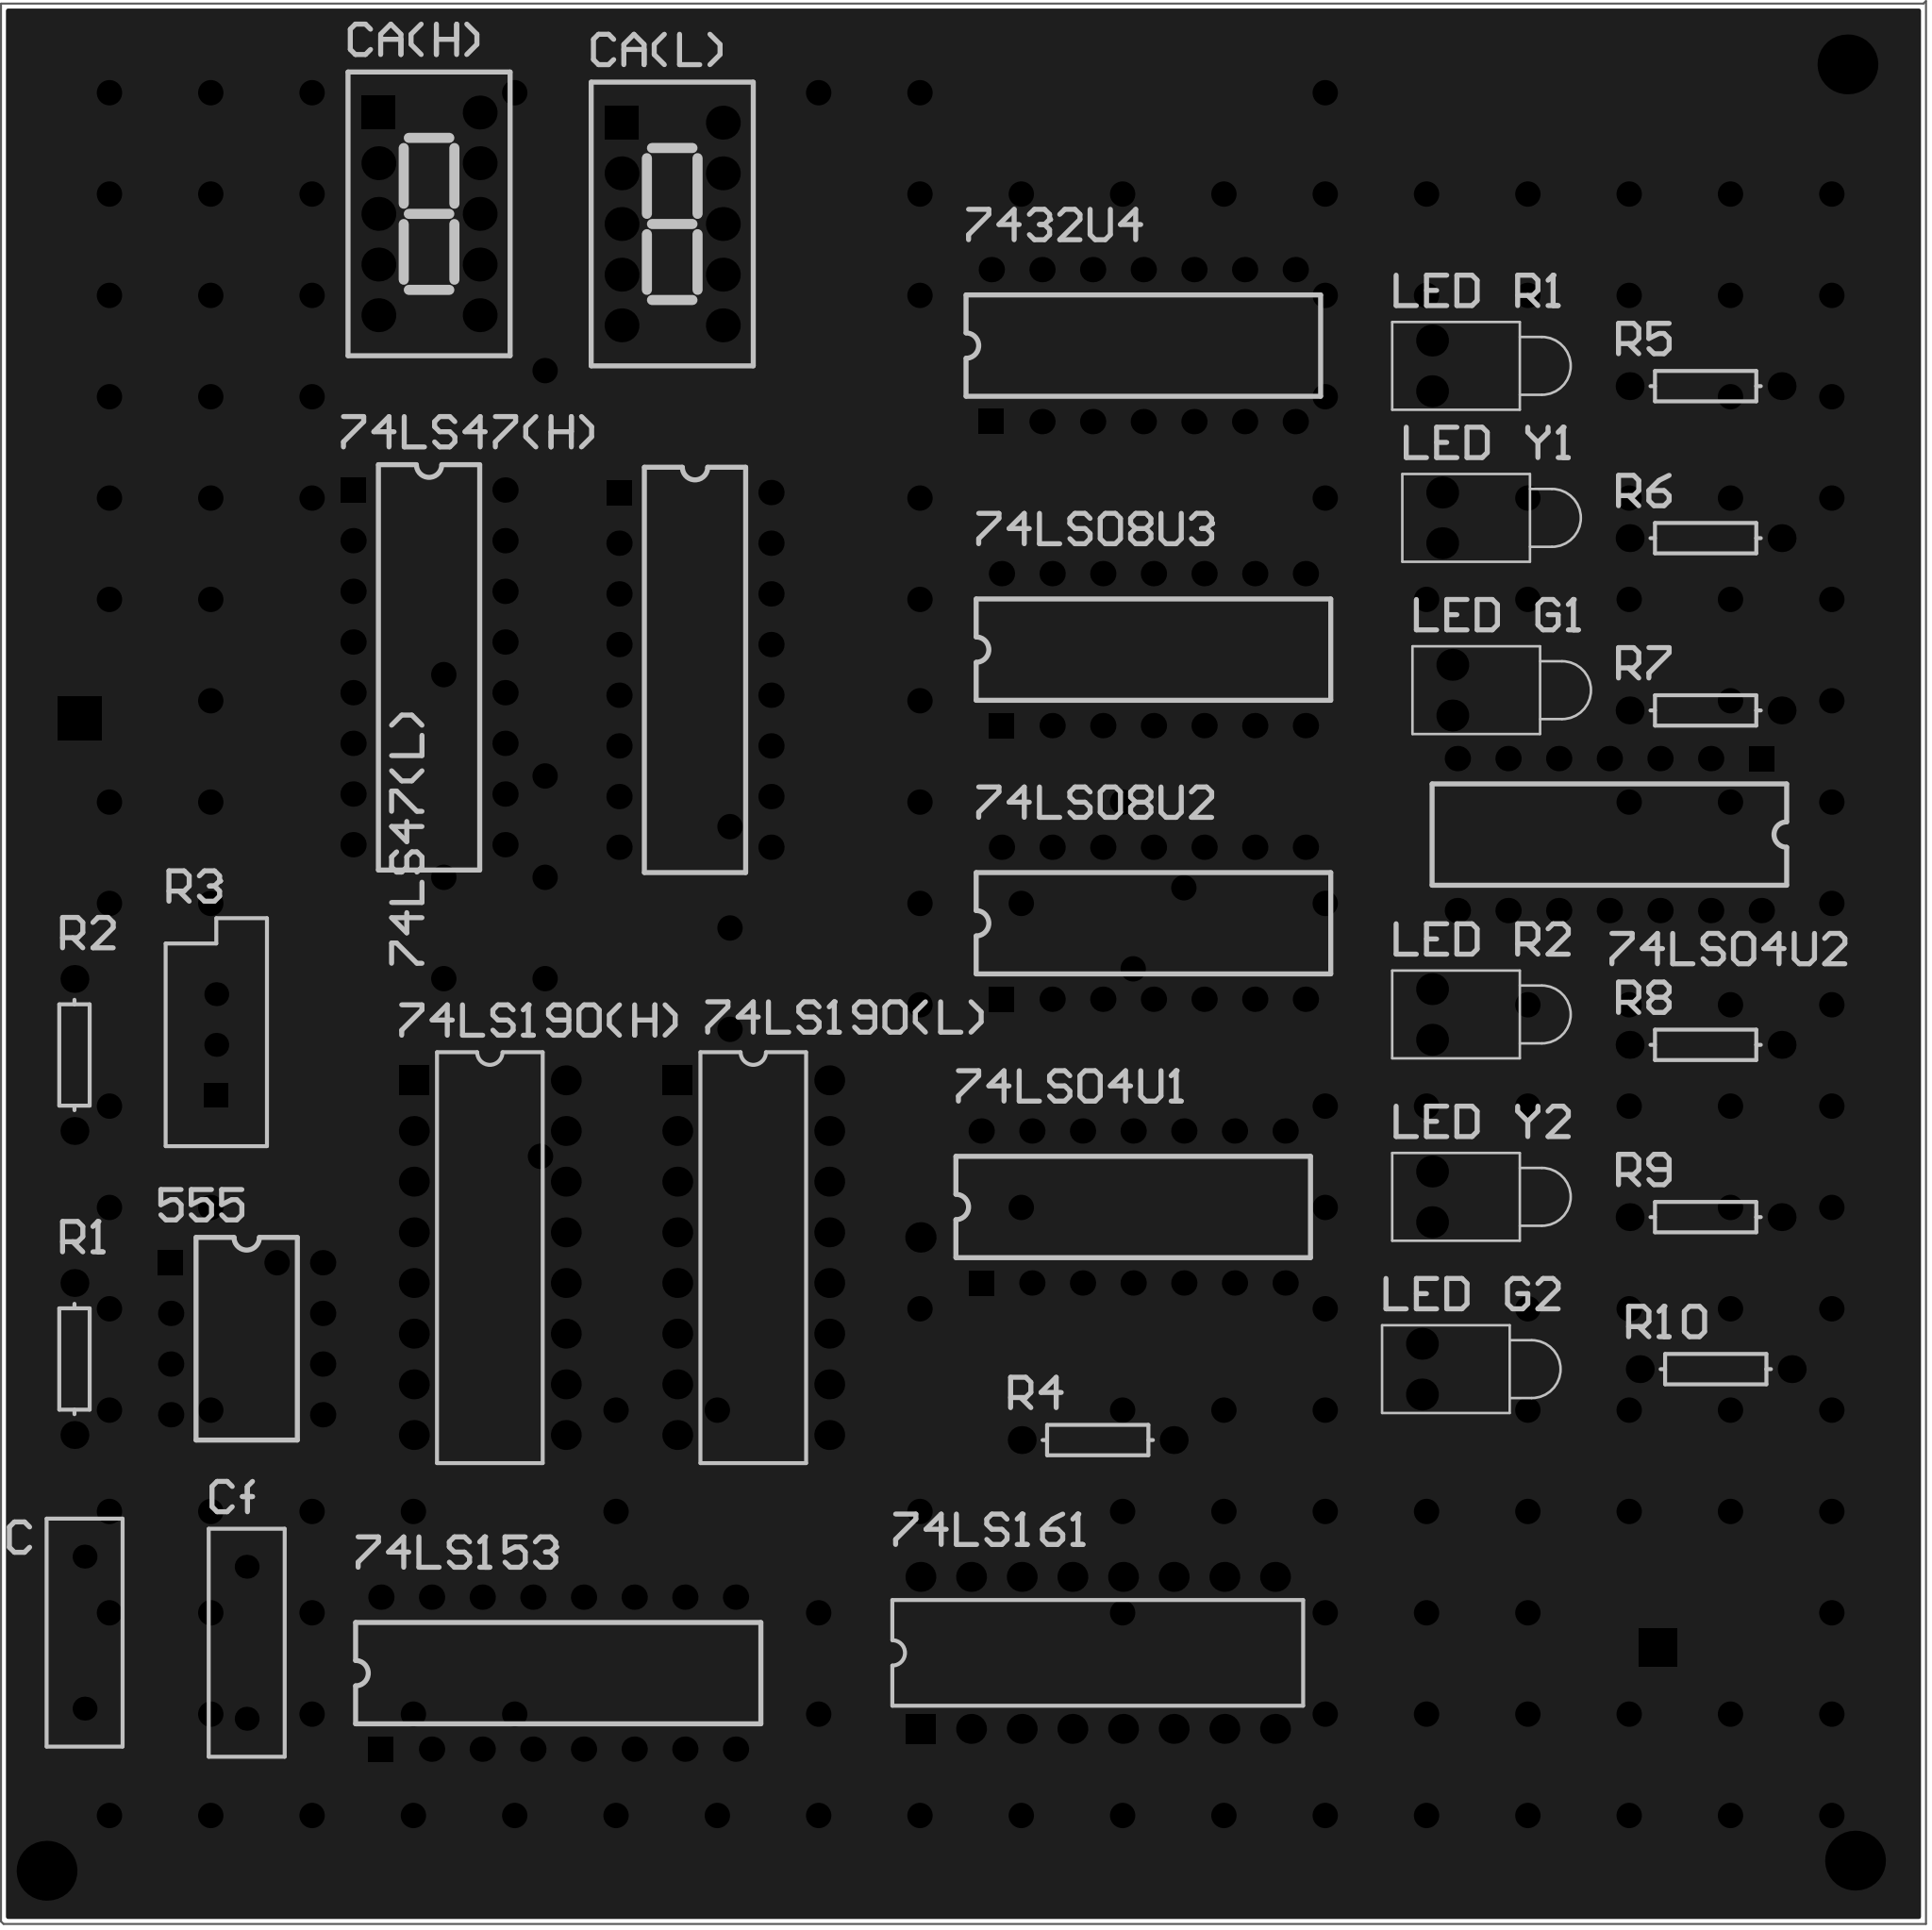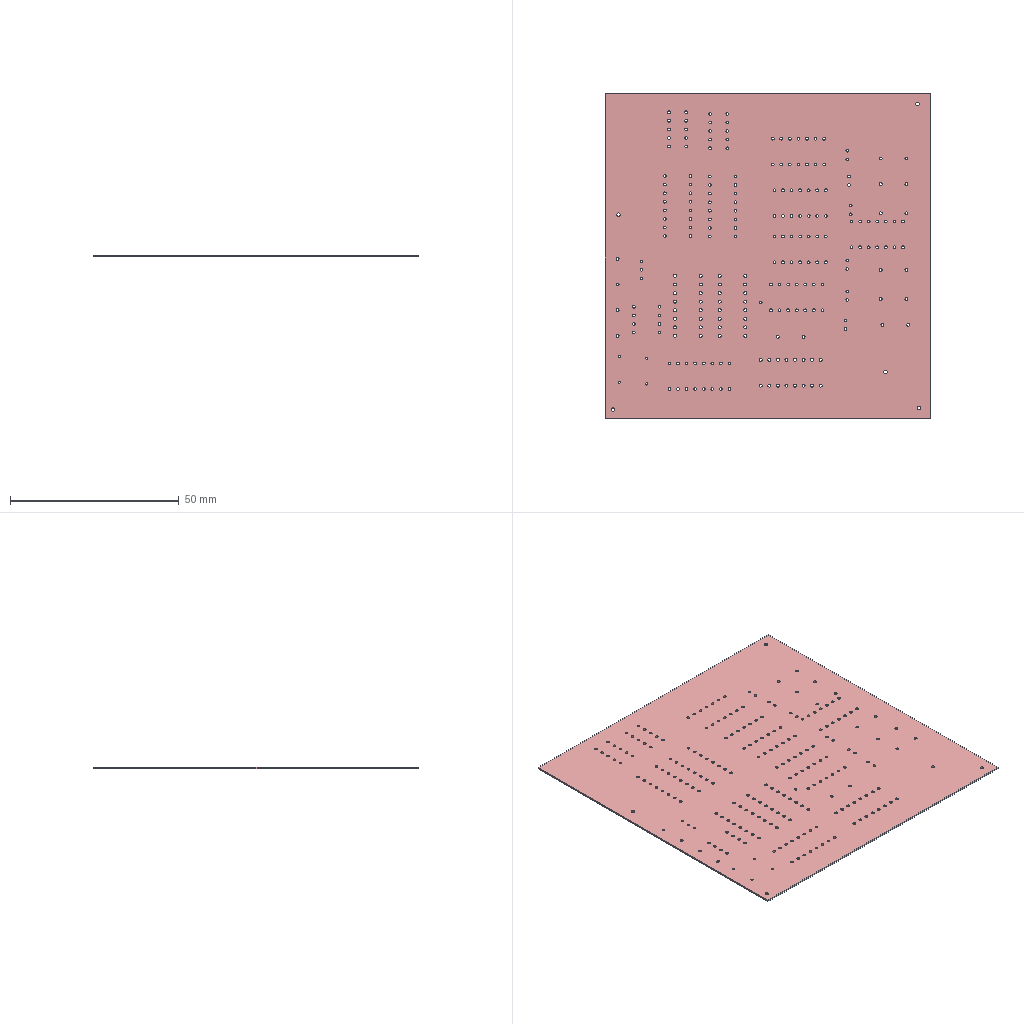Circuit board layout | Altium Designer | box 96.5 x 96.4 x 0.5 mm
Layer stack:
# Altium Designer layer stack of  (unit mm; dielectric type: 0 none, 1 core, 2 prepreg, 3 surface material)
index,name,kind,layer,copper_thickness_mm,dielectric_type,dielectric_thickness_mm,dielectric_material,dielectric_constant
0,Top Paste Mask Layer,other,,,,,,
1,Top Silkscreen Layer,other,,,,,,
2,Top Solder Mask Layer,dielectric,,,3,0.0356,FR-4,4.8
3,Top Layer,copper,Top Layer,0.0356,,,,
4,Substrate1,dielectric,,,3,0.32,FR-4,4.8
5,Bottom Layer,copper,Bottom Layer,0.0356,,,,
6,Bottom Solder Mask Layer,dielectric,,,3,0.0356,FR-4,4.8
7,Bottom Silkscreen Layer,other,,,,,,
8,Bottom Paste Mask Layer,other,,,,,,
# drill layer pairs: low layer,high layer
drill_pair,Top Layer,Bottom Layer
Part placement:
Designator,Comment,Layer,Footprint,Center-X(mm),Center-Y(mm),Rotation
R10,Res1,TopLayer,AXIAL-0.3,172.339,114.3,0
R9,Res1,TopLayer,AXIAL-0.3,171.831,121.92,0
R8,Res1,TopLayer,AXIAL-0.3,171.831,130.556,0
R7,Res1,TopLayer,AXIAL-0.3,171.831,147.32,0
R6,Res1,TopLayer,AXIAL-0.3,171.831,155.956,0
R5,Res1,TopLayer,AXIAL-0.3,171.831,163.576,0
R4,Res1,TopLayer,AXIAL-0.3,141.351,110.744,180
R3,RPot,TopLayer,VR5,97.155,130.556,90
R2,Res1,TopLayer,AXIAL-0.3,90.043,130.048,90
R1,Res1,TopLayer,AXIAL-0.3,90.043,114.808,90
LED Y2,LED1,TopLayer,LED-1,158.115,122.936,0
LED Y1,LED1,TopLayer,LED-1,158.623,156.972,0
LED R2,LED1,TopLayer,LED-1,158.115,132.08,0
LED R1,LED1,TopLayer,LED-1,158.115,164.592,0
LED G2,LED1,TopLayer,LED-1,157.607,114.3,0
LED G1,LED1,TopLayer,LED-1,159.131,148.336,0
C,Cap,TopLayer,RAD-0.3,90.551,101.092,90
Cf,Cap,TopLayer,RAD-0.3,98.679,100.584,90
7432U4,7432,TopLayer,DIP14,143.637,165.608,90
555,555,TopLayer,DIP8,98.679,115.824,0
74LS190(L),SN74LS190,TopLayer,DIP-16,124.079,119.888,270
74LS190(H),SN74LS190,TopLayer,DIP-16,110.871,119.888,270
74LS161,74LS161A,TopLayer,DIP-16,141.351,100.076,0
74LS153,SN74LS153,TopLayer,DIP16,114.3,99.06,90
74LS47(H),SN7447A,TopLayer,DIP16,107.823,149.479,0
74LS08U3,74LS08,TopLayer,DIP14,144.145,150.368,90
74LS08U2,74LS08,TopLayer,DIP14,144.145,136.652,90
74LS04U1,74LS04,TopLayer,DIP14,143.129,122.428,90
74LS04U2,74LS04,TopLayer,DIP14,167.005,141.097,270
74LS47(L),SN7447A,TopLayer,DIP16,121.158,149.352,0
CA(H),Dpy Red-CA,TopLayer,SMG_0.36-1P,107.823,172.212,0
CA(L),Dpy Red-CA,TopLayer,SMG_0.36-1P,120.015,171.704,0
Pad and via stacks:
# Altium Designer via and pad stacks of  (unit mm). Each distinct definition once, with the count of objects using it.
# via: kind,start_layer,end_layer,hole_mm,diameter_mm,mode(0 simple;1 top-mid-bottom;2 full stack),diameter_per_layer,count,example_net
# pad: kind,layer,hole_mm,hole_type(0 round;1 square;2 slot),plating,top_size,top_shape(1 round;2 rect;3 octagon;9 rounded rect),mid_size,bottom_size,mode,footprint,size_per_layer,count,example
pad,Multi-Layer,1,0,plated,1.9x1.9,2,1.9x1.9,1.9x1.9,0,,,1,3
pad,Multi-Layer,1,0,plated,2.2x2.2,2,2.2x2.2,2.2x2.2,0,,,1,2
pad,Multi-Layer,0.762,0,plated,1.524x1.524,1,1.524x1.524,1.524x1.524,0,,,1,1
pad,Multi-Layer,1,0,unplated,3x3,1,3x3,3x3,0,,,3,12
pad,Multi-Layer,0.85,0,plated,1.4x1.4,1,1.4x1.4,1.4x1.4,0,AXIAL-0.3,,18,R10.2
pad,Multi-Layer,0.7,0,plated,1.2x1.2,2,1.2x1.2,1.2x1.2,0,VR5,,1,R3.1
pad,Multi-Layer,0.7,0,plated,1.2x1.2,1,1.2x1.2,1.2x1.2,0,VR5,,2,R3.2
pad,Multi-Layer,0.8,0,plated,1.6x1.6,1,1.6x1.6,1.6x1.6,0,LED-1,,12,LED Y2.1
pad,Multi-Layer,0.7,0,plated,1.2x1.2,1,1.2x1.2,1.2x1.2,0,RAD-0.3,,4,C.2
pad,Multi-Layer,0.8128,0,plated,1.27x1.27,1,1.27x1.27,1.27x1.27,0,DIP14,,65,7432U4.14
pad,Multi-Layer,0.8128,0,plated,1.27x1.27,2,1.27x1.27,1.27x1.27,0,DIP14,,5,7432U4.1
pad,Multi-Layer,0.8128,0,plated,1.27x1.27,2,1.27x1.27,1.27x1.27,0,DIP8,,1,555.1
pad,Multi-Layer,0.8128,0,plated,1.27x1.27,1,1.27x1.27,1.27x1.27,0,DIP8,,7,555.2
pad,Multi-Layer,0.9,0,plated,1.5x1.5,1,1.5x1.5,1.5x1.5,0,DIP-16,,45,74LS190(L).9
pad,Multi-Layer,0.9,0,plated,1.5x1.5,2,1.5x1.5,1.5x1.5,0,DIP-16,,3,74LS190(L).1
pad,Multi-Layer,0.8128,0,plated,1.27x1.27,2,1.27x1.27,1.27x1.27,0,DIP16,,3,74LS153.1
pad,Multi-Layer,0.8128,0,plated,1.27x1.27,1,1.27x1.27,1.27x1.27,0,DIP16,,45,74LS153.2
pad,Multi-Layer,0.8,0,plated,1.7x1.7,1,1.7x1.7,1.7x1.7,0,SMG 0.36-1P,,18,CA(H).10
pad,Multi-Layer,0.8,0,plated,1.7x1.7,2,1.7x1.7,1.7x1.7,0,SMG 0.36-1P,,2,CA(H).1
via,Top Layer,Bottom Layer,0.7112,1.27,0,,172,$2N1342
Copper pours:
name,layer,net,type(0 solid;1 hatched;2 none)
Top Layer-GND,Top Layer,GND,0
Bottom Layer-GND,Bottom Layer,GND,0
Design rules, without the lines most boards share:
# Altium Designer design rules of  (exported by Altium Designer, unit mm)
# columns: name | kind | enabled | priority | scope1 | scope2 | descriptor | typed fields (field=value)
ComponentClearance_1 | 24 | enabled | 1 | All | All | Component Clearance Constraint ( Horizontal Gap = 10mil, Vertical Gap = 10mil ) (All),(All)  | gap=0.254
Plane_PlaneConnect | 0 | disabled | 1 | All | All | Clearance Constraint (Gap=10mil) (Disabled)(All),(All) | gap=0.254
Plane_PlaneConnect_1 | 63 | disabled | 1 | All | All | Board Clearance Constraint (Gap=0mil) (Disabled)(All) |
Copper_PolygonConnect | 0 | disabled | 2 | All | All | Clearance Constraint (Gap=10mil) (Disabled)(All),(All) | gap=0.254
Copper_PolygonConnect_1 | 63 | disabled | 2 | All | All | Board Clearance Constraint (Gap=0mil) (Disabled)(All) |
Clearance | 0 | enabled | 3 | All | All | Clearance Constraint (Gap=10mil) (All),(All) | gap=0.254
Clearance_1 | 63 | enabled | 3 | All | All | Board Clearance Constraint (Gap=0mil) (All) |
ComponentClearance | 52 | enabled | 1 | All | All | Hole To Hole Clearance (Gap=10mil) (All),(All) | gap=0.254
Width | 2 | enabled | 1 | All | All | Width Constraint (Min=10mil) (Max=10mil) (Preferred=10mil) (All) |
DiffPairsRouting | 51 | enabled | 1 | All | All | Differential Pairs Uncoupled Length using the Gap Constraints (Min=10mil) (Max=10mil) (Prefered=10mil)  and Width Constraints (Min=99999mil) (Max=0mil) (Prefered=0mil) (All) |
RoutingVias | 11 | enabled | 1 | All | All | Routing Via (MinHoleWidth=28mil) (MaxHoleWidth=28mil) (PreferredHoleWidth=28mil) (MinWidth=50mil) (MaxWidth=50mil) (PreferedWidth=50mil) (All) | via_min_hole=0.7112 via_max_hole=0.7112 via_preferred_diameter=1.27 via_preferred_hole=0.7112
PlaneConnect | 6 | enabled | 1 | All | All | Power Plane Connect Rule(Relief Connect )(Expansion=20mil) (Conductor Width=10mil) (Air Gap=10mil) (Entries=4) (All) | relief_conductor_width=0.254 relief_entries=4 relief_expansion=0.508
PolygonConnect | 20 | enabled | 1 | (InNet('GND')) | All | Polygon Connect Rule(Relief Connect )(Conductor Width=10mil) (Relief Angle=90 Angle) (Entries=4) (Air Gap Width=10mil) ((InNet('GND'))),(All) | connect_style(0=relief,1=direct,2=none)=0 relief_conductor_width=0.254 relief_entries=4
PasteMaskExpansion | 14 | enabled | 1 | All | All | Paste Mask Expansion (Expansion =0mil) (All) | expansion=0
SolderMaskExpansion | 13 | enabled | 1 | All | All | Solder Mask Expansion (Expansion =4mil) (All) | expansion=0.1016